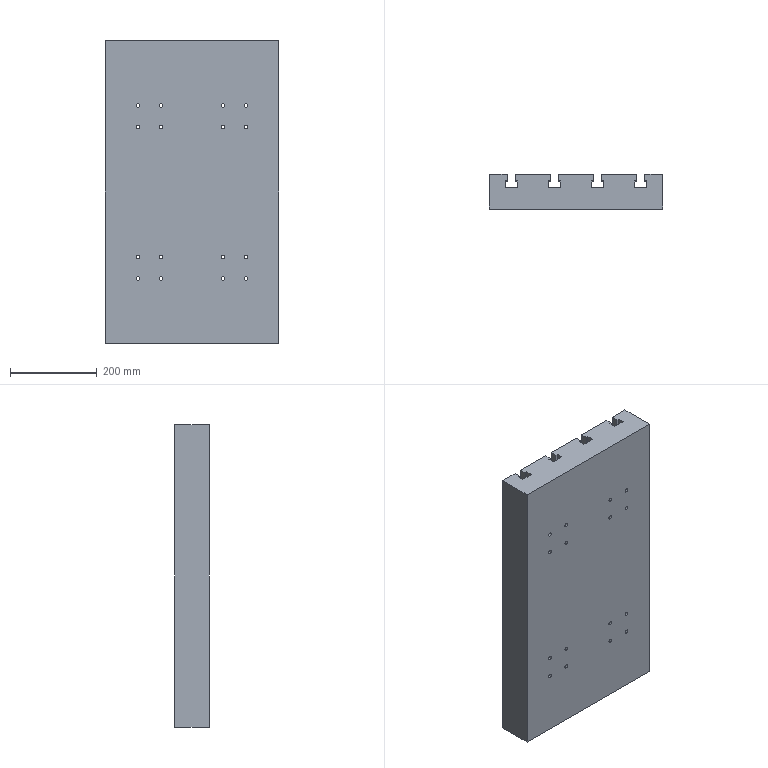Part | SolidWorks | features BaseBody 1 | 1 solid | 146 faces | box 400 x 80 x 700 mm | volume 20359405 mm3 | cylinder 80 | plane 58 | cone 8 | commonest cylinder face diameters 8.4 x32 15 x32 11 x8 21.48 x8